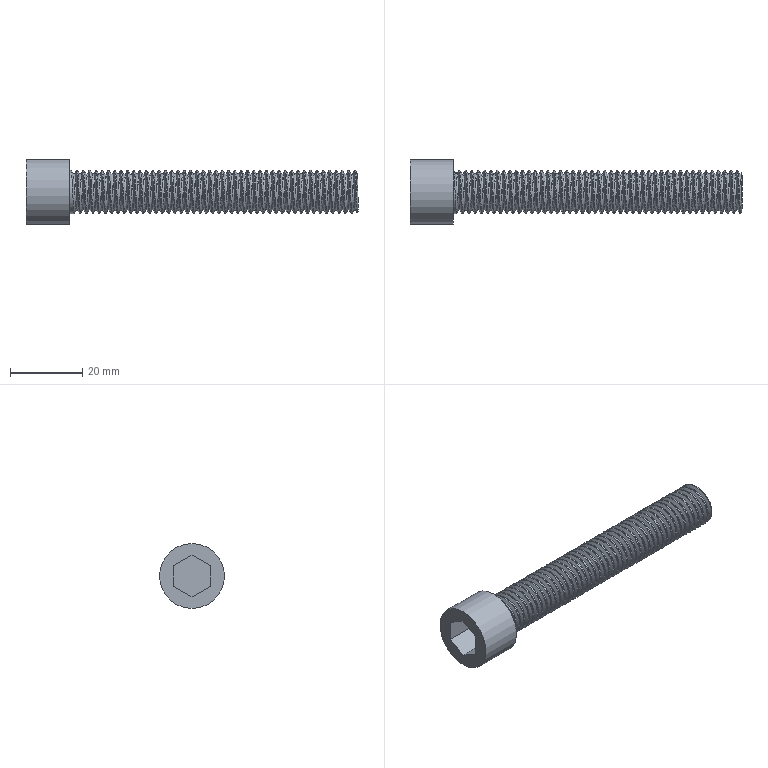Part | STEP file | Tube feed_id458_x_t | 1 solid | 18 faces | box 92 x 18 x 18 mm | volume 10186 mm3 | plane 11 | cylinder 3 | spline 3 | cone 1 | commonest cylinder face diameters 10.25 x1 12 x1 18 x1